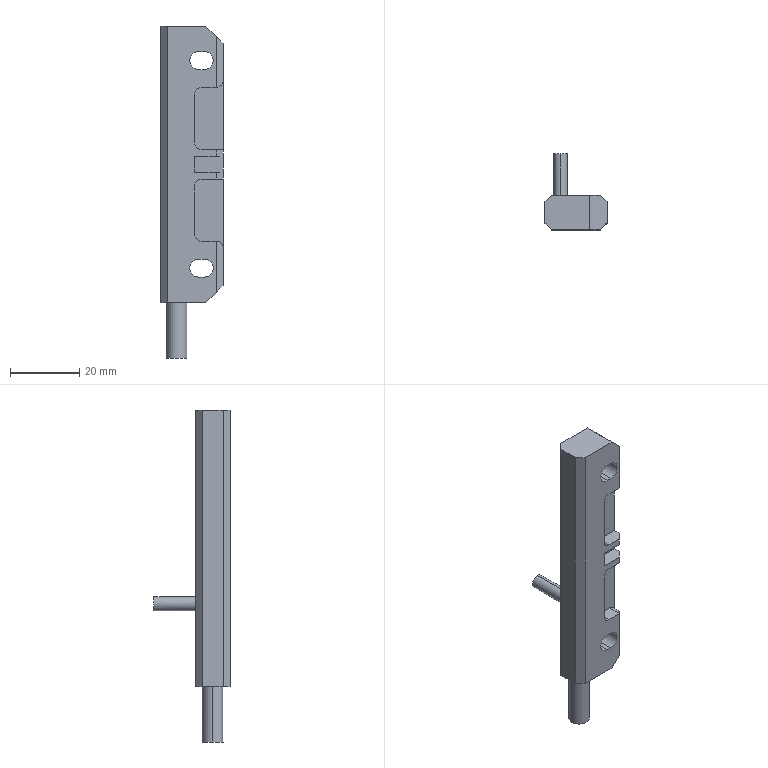Part | STEP file | 001-001-hfy44-96-r | 3 solids | 108 faces | box 18 x 22 x 96 mm | volume 10397 mm3 | plane 56 | cylinder 29 | torus 23 | commonest cylinder face diameters 4 x14 6 x6 5.2 x4 4.5 x3 5 x2